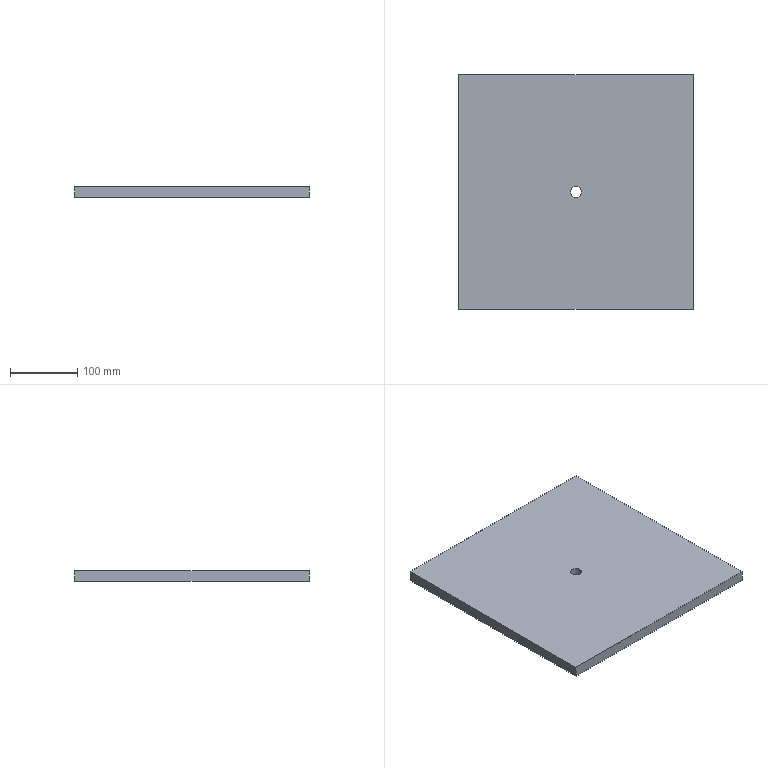Part | SolidWorks | features BaseBody 1 | 1 solid | 8 faces | box 350 x 350 x 16 mm | volume 1956783 mm3 | plane 6 | cylinder 2 | commonest cylinder face diameters 16 x2
STEP:
#1=CARTESIAN_POINT('',(298.547,1729.544,-1224.));
#2=VERTEX_POINT('',#1);
#3=CARTESIAN_POINT('',(282.547,1729.544,-1224.));
#4=VERTEX_POINT('',#3);
#5=CARTESIAN_POINT('',(290.547,1729.544,-1224.));
#6=DIRECTION('',(0.,0.,-1.));
#7=DIRECTION('',(1.,0.,0.));
#8=AXIS2_PLACEMENT_3D('',#5,#6,#7);
#9=CIRCLE('',#8,8.);
#10=EDGE_CURVE('',#2,#4,#9,.T.);
#11=ORIENTED_EDGE('',*,*,#10,.T.);
#12=CARTESIAN_POINT('',(282.547,1729.544,-1208.));
#13=VERTEX_POINT('',#12);
#14=CARTESIAN_POINT('',(282.547,1729.544,-1246.627));
#15=DIRECTION('',(0.,0.,1.));
#16=VECTOR('',#15,1000.);
#17=LINE('',#14,#16);
#18=EDGE_CURVE('',#4,#13,#17,.T.);
#19=ORIENTED_EDGE('',*,*,#18,.T.);
#20=CARTESIAN_POINT('',(298.547,1729.544,-1208.));
#21=VERTEX_POINT('',#20);
#22=CARTESIAN_POINT('',(290.547,1729.544,-1208.));
#23=DIRECTION('',(0.,0.,-1.));
#24=DIRECTION('',(1.,0.,0.));
#25=AXIS2_PLACEMENT_3D('',#22,#23,#24);
#26=CIRCLE('',#25,8.);
#27=EDGE_CURVE('',#21,#13,#26,.T.);
#28=ORIENTED_EDGE('',*,*,#27,.F.);
#29=CARTESIAN_POINT('',(298.547,1729.544,-1246.627));
#30=DIRECTION('',(0.,0.,1.));
#31=VECTOR('',#30,1000.);
#32=LINE('',#29,#31);
#33=EDGE_CURVE('',#2,#21,#32,.T.);
#34=ORIENTED_EDGE('',*,*,#33,.F.);
#35=EDGE_LOOP('',(#11,#19,#28,#34));
#36=FACE_OUTER_BOUND('',#35,.T.);
#37=CARTESIAN_POINT('',(290.547,1729.544,-1246.627));
#38=DIRECTION('',(0.,0.,1.));
#39=DIRECTION('',(1.,0.,0.));
#40=AXIS2_PLACEMENT_3D('',#37,#38,#39);
#41=CYLINDRICAL_SURFACE('',#40,8.);
#42=ADVANCED_FACE('',(#36),#41,.F.);
#43=ORIENTED_EDGE('',*,*,#10,.F.);
#44=CARTESIAN_POINT('',(290.547,1729.544,-1224.));
#45=DIRECTION('',(0.,0.,-1.));
#46=DIRECTION('',(1.,0.,0.));
#47=AXIS2_PLACEMENT_3D('',#44,#45,#46);
#48=CIRCLE('',#47,8.);
#49=EDGE_CURVE('',#4,#2,#48,.T.);
#50=ORIENTED_EDGE('',*,*,#49,.F.);
#51=EDGE_LOOP('',(#43,#50));
#52=FACE_BOUND('',#51,.T.);
#53=CARTESIAN_POINT('',(465.547,1904.544,-1224.));
#54=VERTEX_POINT('',#53);
#55=CARTESIAN_POINT('',(115.547,1904.544,-1224.));
#56=VERTEX_POINT('',#55);
#57=CARTESIAN_POINT('',(115.547,1904.544,-1224.));
#58=DIRECTION('',(-1.,0.,0.));
#59=VECTOR('',#58,1000.);
#60=LINE('',#57,#59);
#61=EDGE_CURVE('',#54,#56,#60,.T.);
#62=ORIENTED_EDGE('',*,*,#61,.F.);
#63=CARTESIAN_POINT('',(465.547,1554.544,-1224.));
#64=VERTEX_POINT('',#63);
#65=CARTESIAN_POINT('',(465.547,1554.544,-1224.));
#66=DIRECTION('',(0.,1.,0.));
#67=VECTOR('',#66,1000.);
#68=LINE('',#65,#67);
#69=EDGE_CURVE('',#64,#54,#68,.T.);
#70=ORIENTED_EDGE('',*,*,#69,.F.);
#71=CARTESIAN_POINT('',(115.547,1554.544,-1224.));
#72=VERTEX_POINT('',#71);
#73=CARTESIAN_POINT('',(115.547,1554.544,-1224.));
#74=DIRECTION('',(1.,0.,0.));
#75=VECTOR('',#74,1000.);
#76=LINE('',#73,#75);
#77=EDGE_CURVE('',#72,#64,#76,.T.);
#78=ORIENTED_EDGE('',*,*,#77,.F.);
#79=CARTESIAN_POINT('',(115.547,1554.544,-1224.));
#80=DIRECTION('',(0.,-1.,0.));
#81=VECTOR('',#80,1000.);
#82=LINE('',#79,#81);
#83=EDGE_CURVE('',#56,#72,#82,.T.);
#84=ORIENTED_EDGE('',*,*,#83,.F.);
#85=EDGE_LOOP('',(#62,#70,#78,#84));
#86=FACE_OUTER_BOUND('',#85,.T.);
#87=CARTESIAN_POINT('',(115.547,1554.544,-1224.));
#88=DIRECTION('',(0.,0.,1.));
#89=DIRECTION('',(1.,0.,0.));
#90=AXIS2_PLACEMENT_3D('',#87,#88,#89);
#91=PLANE('',#90);
#92=ADVANCED_FACE('',(#52,#86),#91,.F.);
#93=ORIENTED_EDGE('',*,*,#18,.F.);
#94=ORIENTED_EDGE('',*,*,#49,.T.);
#95=ORIENTED_EDGE('',*,*,#33,.T.);
#96=CARTESIAN_POINT('',(290.547,1729.544,-1208.));
#97=DIRECTION('',(0.,0.,-1.));
#98=DIRECTION('',(1.,0.,0.));
#99=AXIS2_PLACEMENT_3D('',#96,#97,#98);
#100=CIRCLE('',#99,8.);
#101=EDGE_CURVE('',#13,#21,#100,.T.);
#102=ORIENTED_EDGE('',*,*,#101,.F.);
#103=EDGE_LOOP('',(#93,#94,#95,#102));
#104=FACE_OUTER_BOUND('',#103,.T.);
#105=CARTESIAN_POINT('',(290.547,1729.544,-1246.627));
#106=DIRECTION('',(0.,0.,1.));
#107=DIRECTION('',(1.,0.,0.));
#108=AXIS2_PLACEMENT_3D('',#105,#106,#107);
#109=CYLINDRICAL_SURFACE('',#108,8.);
#110=ADVANCED_FACE('',(#104),#109,.F.);
#111=CARTESIAN_POINT('',(115.547,1904.544,-1208.));
#112=VERTEX_POINT('',#111);
#113=CARTESIAN_POINT('',(115.547,1554.544,-1208.));
#114=VERTEX_POINT('',#113);
#115=CARTESIAN_POINT('',(115.547,1904.544,-1208.));
#116=DIRECTION('',(0.,-1.,0.));
#117=VECTOR('',#116,1000.);
#118=LINE('',#115,#117);
#119=EDGE_CURVE('',#112,#114,#118,.T.);
#120=ORIENTED_EDGE('',*,*,#119,.F.);
#121=CARTESIAN_POINT('',(115.547,1904.544,-1208.));
#122=DIRECTION('',(0.,0.,1.));
#123=VECTOR('',#122,1000.);
#124=LINE('',#121,#123);
#125=EDGE_CURVE('',#56,#112,#124,.T.);
#126=ORIENTED_EDGE('',*,*,#125,.F.);
#127=ORIENTED_EDGE('',*,*,#83,.T.);
#128=CARTESIAN_POINT('',(115.547,1554.544,-1208.));
#129=DIRECTION('',(0.,0.,-1.));
#130=VECTOR('',#129,1000.);
#131=LINE('',#128,#130);
#132=EDGE_CURVE('',#114,#72,#131,.T.);
#133=ORIENTED_EDGE('',*,*,#132,.F.);
#134=EDGE_LOOP('',(#120,#126,#127,#133));
#135=FACE_OUTER_BOUND('',#134,.T.);
#136=CARTESIAN_POINT('',(115.547,1904.544,-1208.));
#137=DIRECTION('',(1.,0.,0.));
#138=DIRECTION('',(0.,0.,-1.));
#139=AXIS2_PLACEMENT_3D('',#136,#137,#138);
#140=PLANE('',#139);
#141=ADVANCED_FACE('',(#135),#140,.F.);
#142=CARTESIAN_POINT('',(465.547,1904.544,-1208.));
#143=VERTEX_POINT('',#142);
#144=CARTESIAN_POINT('',(185.547,1904.544,-1208.));
#145=DIRECTION('',(-1.,0.,0.));
#146=VECTOR('',#145,1000.);
#147=LINE('',#144,#146);
#148=EDGE_CURVE('',#143,#112,#147,.T.);
#149=ORIENTED_EDGE('',*,*,#148,.F.);
#150=CARTESIAN_POINT('',(465.547,1904.544,-1208.));
#151=DIRECTION('',(0.,0.,1.));
#152=VECTOR('',#151,1000.);
#153=LINE('',#150,#152);
#154=EDGE_CURVE('',#54,#143,#153,.T.);
#155=ORIENTED_EDGE('',*,*,#154,.F.);
#156=ORIENTED_EDGE('',*,*,#61,.T.);
#157=ORIENTED_EDGE('',*,*,#125,.T.);
#158=EDGE_LOOP('',(#149,#155,#156,#157));
#159=FACE_OUTER_BOUND('',#158,.T.);
#160=CARTESIAN_POINT('',(185.547,1904.544,-1208.));
#161=DIRECTION('',(0.,-1.,0.));
#162=DIRECTION('',(0.,0.,-1.));
#163=AXIS2_PLACEMENT_3D('',#160,#161,#162);
#164=PLANE('',#163);
#165=ADVANCED_FACE('',(#159),#164,.F.);
#166=CARTESIAN_POINT('',(465.547,1554.544,-1208.));
#167=VERTEX_POINT('',#166);
#168=CARTESIAN_POINT('',(465.547,1904.544,-1208.));
#169=DIRECTION('',(0.,1.,0.));
#170=VECTOR('',#169,1000.);
#171=LINE('',#168,#170);
#172=EDGE_CURVE('',#167,#143,#171,.T.);
#173=ORIENTED_EDGE('',*,*,#172,.F.);
#174=CARTESIAN_POINT('',(465.547,1554.544,-1208.));
#175=DIRECTION('',(0.,0.,1.));
#176=VECTOR('',#175,1000.);
#177=LINE('',#174,#176);
#178=EDGE_CURVE('',#64,#167,#177,.T.);
#179=ORIENTED_EDGE('',*,*,#178,.F.);
#180=ORIENTED_EDGE('',*,*,#69,.T.);
#181=ORIENTED_EDGE('',*,*,#154,.T.);
#182=EDGE_LOOP('',(#173,#179,#180,#181));
#183=FACE_OUTER_BOUND('',#182,.T.);
#184=CARTESIAN_POINT('',(465.547,1904.544,-1208.));
#185=DIRECTION('',(-1.,0.,0.));
#186=DIRECTION('',(0.,0.,1.));
#187=AXIS2_PLACEMENT_3D('',#184,#185,#186);
#188=PLANE('',#187);
#189=ADVANCED_FACE('',(#183),#188,.F.);
#190=CARTESIAN_POINT('',(465.547,1554.544,-1208.));
#191=DIRECTION('',(1.,0.,0.));
#192=VECTOR('',#191,1000.);
#193=LINE('',#190,#192);
#194=EDGE_CURVE('',#114,#167,#193,.T.);
#195=ORIENTED_EDGE('',*,*,#194,.F.);
#196=ORIENTED_EDGE('',*,*,#132,.T.);
#197=ORIENTED_EDGE('',*,*,#77,.T.);
#198=ORIENTED_EDGE('',*,*,#178,.T.);
#199=EDGE_LOOP('',(#195,#196,#197,#198));
#200=FACE_OUTER_BOUND('',#199,.T.);
#201=CARTESIAN_POINT('',(465.547,1554.544,-1208.));
#202=DIRECTION('',(0.,1.,0.));
#203=DIRECTION('',(0.,0.,1.));
#204=AXIS2_PLACEMENT_3D('',#201,#202,#203);
#205=PLANE('',#204);
#206=ADVANCED_FACE('',(#200),#205,.F.);
#207=ORIENTED_EDGE('',*,*,#27,.T.);
#208=ORIENTED_EDGE('',*,*,#101,.T.);
#209=EDGE_LOOP('',(#207,#208));
#210=FACE_BOUND('',#209,.T.);
#211=ORIENTED_EDGE('',*,*,#119,.T.);
#212=ORIENTED_EDGE('',*,*,#194,.T.);
#213=ORIENTED_EDGE('',*,*,#172,.T.);
#214=ORIENTED_EDGE('',*,*,#148,.T.);
#215=EDGE_LOOP('',(#211,#212,#213,#214));
#216=FACE_OUTER_BOUND('',#215,.T.);
#217=CARTESIAN_POINT('',(115.547,1554.544,-1208.));
#218=DIRECTION('',(0.,0.,1.));
#219=DIRECTION('',(1.,0.,0.));
#220=AXIS2_PLACEMENT_3D('',#217,#218,#219);
#221=PLANE('',#220);
#222=ADVANCED_FACE('',(#210,#216),#221,.T.);
#223=CLOSED_SHELL('',(#42,#92,#110,#141,#165,#189,#206,#222));
#224=MANIFOLD_SOLID_BREP('',#223);
#225=CARTESIAN_POINT('',(0.,0.,0.));
#226=DIRECTION('',(0.,0.,1.));
#227=DIRECTION('',(1.,0.,0.));
#228=AXIS2_PLACEMENT_3D('',#225,#226,#227);
#229=(LENGTH_UNIT()NAMED_UNIT(*)SI_UNIT(.MILLI.,.METRE.));
#230=UNCERTAINTY_MEASURE_WITH_UNIT(LENGTH_MEASURE(0.00001),#229,'','');
#231=(NAMED_UNIT(*)PLANE_ANGLE_UNIT()SI_UNIT($,.RADIAN.));
#232=(NAMED_UNIT(*)SI_UNIT($,.STERADIAN.)SOLID_ANGLE_UNIT());
#233=(GEOMETRIC_REPRESENTATION_CONTEXT(3)GLOBAL_UNCERTAINTY_ASSIGNED_CONTEXT((#230))GLOBAL_UNIT_ASSIGNED_CONTEXT((#229,#231,#232))REPRESENTATION_CONTEXT('',''));
#234=ADVANCED_BREP_SHAPE_REPRESENTATION('',(#224,#228),#233);